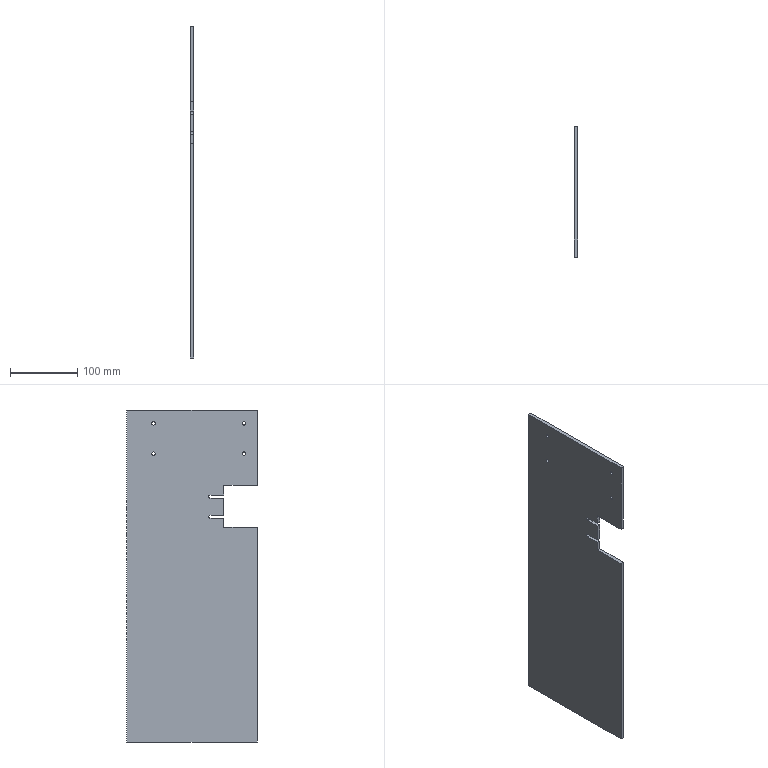Part | STEP file | 09-11 Outer side plate 4 | 1 solid | 26 faces | box 5 x 195 x 495 mm | volume 465621 mm3 | plane 16 | cylinder 10 | commonest cylinder face diameters 5 x8 4.705 x2